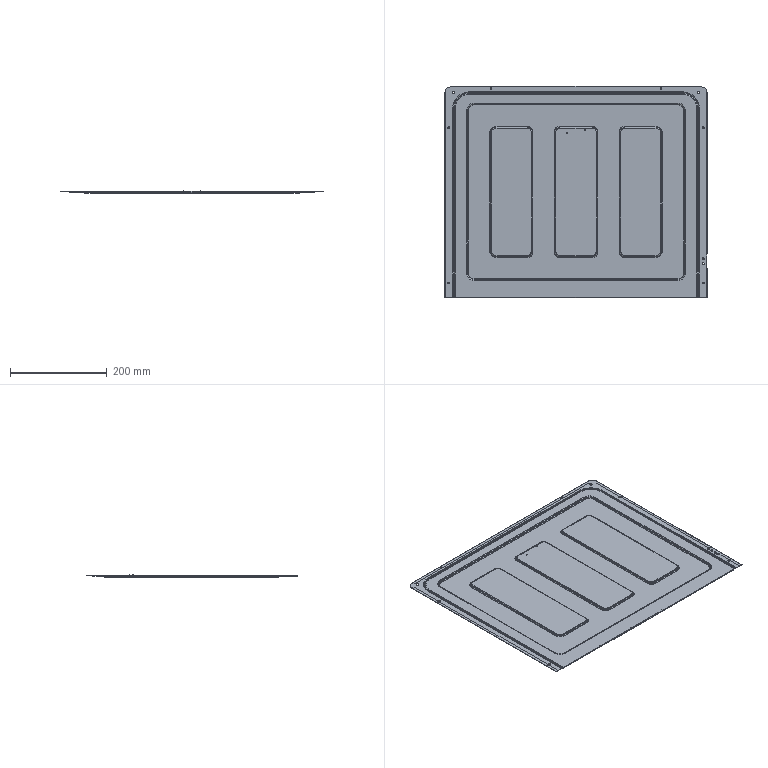Part | STEP file | ZXW722-L-02 | 1 solid | 392 faces | box 540.8 x 435.4 x 4.2 mm | volume 101202 mm3 | cylinder 146 | plane 138 | torus 52 | spline 40 | cone 16 | commonest cylinder face diameters 3 x32 3.8 x32 2 x13 20 x10 4 x8 5 x8